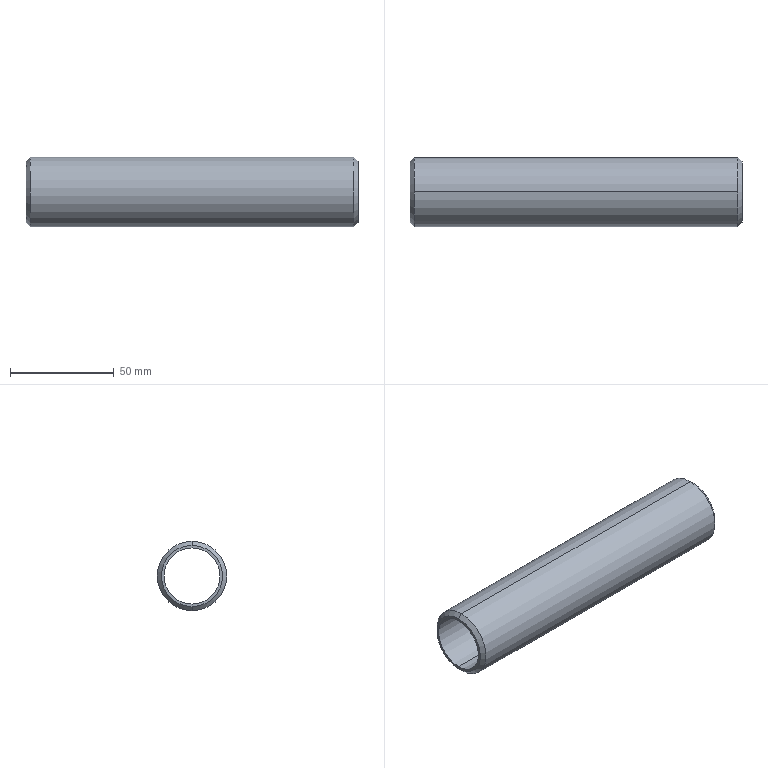Part | SolidWorks | features Chamfer 1, ExtruThin 1 | 1 solid | 10 faces | box 160 x 33.5 x 33.5 mm | volume 49013 mm3 | cone 4 | cylinder 4 | plane 2 | commonest cylinder face diameters 27 x2 33.5 x2
STEP:
#1=CARTESIAN_POINT('',(0.,0.,14.75));
#2=VERTEX_POINT('',#1);
#3=CARTESIAN_POINT('',(0.,0.,-14.75));
#4=VERTEX_POINT('',#3);
#5=CARTESIAN_POINT('',(0.,0.,0.));
#6=DIRECTION('',(-1.,0.,0.));
#7=DIRECTION('',(0.,0.,-1.));
#8=AXIS2_PLACEMENT_3D('',#5,#6,#7);
#9=CIRCLE('',#8,14.75);
#10=EDGE_CURVE('',#2,#4,#9,.T.);
#11=ORIENTED_EDGE('',*,*,#10,.F.);
#12=CARTESIAN_POINT('',(2.,0.,16.75));
#13=VERTEX_POINT('',#12);
#14=CARTESIAN_POINT('',(2.,0.,16.75));
#15=DIRECTION('',(0.7071,0.,0.7071));
#16=VECTOR('',#15,1000.);
#17=LINE('',#14,#16);
#18=EDGE_CURVE('',#2,#13,#17,.T.);
#19=ORIENTED_EDGE('',*,*,#18,.T.);
#20=CARTESIAN_POINT('',(2.,0.,-16.75));
#21=VERTEX_POINT('',#20);
#22=CARTESIAN_POINT('',(2.,0.,0.));
#23=DIRECTION('',(1.,0.,0.));
#24=DIRECTION('',(0.,0.,-1.));
#25=AXIS2_PLACEMENT_3D('',#22,#23,#24);
#26=CIRCLE('',#25,16.75);
#27=EDGE_CURVE('',#21,#13,#26,.T.);
#28=ORIENTED_EDGE('',*,*,#27,.F.);
#29=CARTESIAN_POINT('',(2.,0.,-16.75));
#30=DIRECTION('',(0.7071,0.,-0.7071));
#31=VECTOR('',#30,1000.);
#32=LINE('',#29,#31);
#33=EDGE_CURVE('',#4,#21,#32,.T.);
#34=ORIENTED_EDGE('',*,*,#33,.F.);
#35=EDGE_LOOP('',(#11,#19,#28,#34));
#36=FACE_OUTER_BOUND('',#35,.T.);
#37=CARTESIAN_POINT('',(2.,0.,0.));
#38=DIRECTION('',(1.,0.,0.));
#39=DIRECTION('',(0.,0.,-1.));
#40=AXIS2_PLACEMENT_3D('',#37,#38,#39);
#41=CONICAL_SURFACE('',#40,16.75,0.7854);
#42=ADVANCED_FACE('',(#36),#41,.T.);
#43=CARTESIAN_POINT('',(160.,0.,-14.75));
#44=VERTEX_POINT('',#43);
#45=CARTESIAN_POINT('',(160.,0.,14.75));
#46=VERTEX_POINT('',#45);
#47=CARTESIAN_POINT('',(160.,0.,0.));
#48=DIRECTION('',(1.,0.,0.));
#49=DIRECTION('',(0.,0.,-1.));
#50=AXIS2_PLACEMENT_3D('',#47,#48,#49);
#51=CIRCLE('',#50,14.75);
#52=EDGE_CURVE('',#44,#46,#51,.T.);
#53=ORIENTED_EDGE('',*,*,#52,.F.);
#54=CARTESIAN_POINT('',(158.,0.,-16.75));
#55=VERTEX_POINT('',#54);
#56=CARTESIAN_POINT('',(160.,0.,-14.75));
#57=DIRECTION('',(-0.7071,0.,-0.7071));
#58=VECTOR('',#57,1000.);
#59=LINE('',#56,#58);
#60=EDGE_CURVE('',#44,#55,#59,.T.);
#61=ORIENTED_EDGE('',*,*,#60,.T.);
#62=CARTESIAN_POINT('',(158.,0.,16.75));
#63=VERTEX_POINT('',#62);
#64=CARTESIAN_POINT('',(158.,0.,0.));
#65=DIRECTION('',(-1.,0.,0.));
#66=DIRECTION('',(0.,0.,-1.));
#67=AXIS2_PLACEMENT_3D('',#64,#65,#66);
#68=CIRCLE('',#67,16.75);
#69=EDGE_CURVE('',#63,#55,#68,.T.);
#70=ORIENTED_EDGE('',*,*,#69,.F.);
#71=CARTESIAN_POINT('',(160.,0.,14.75));
#72=DIRECTION('',(-0.7071,0.,0.7071));
#73=VECTOR('',#72,1000.);
#74=LINE('',#71,#73);
#75=EDGE_CURVE('',#46,#63,#74,.T.);
#76=ORIENTED_EDGE('',*,*,#75,.F.);
#77=EDGE_LOOP('',(#53,#61,#70,#76));
#78=FACE_OUTER_BOUND('',#77,.T.);
#79=CARTESIAN_POINT('',(160.,0.,0.));
#80=DIRECTION('',(-1.,0.,0.));
#81=DIRECTION('',(0.,0.,1.));
#82=AXIS2_PLACEMENT_3D('',#79,#80,#81);
#83=CONICAL_SURFACE('',#82,14.75,0.7854);
#84=ADVANCED_FACE('',(#78),#83,.T.);
#85=CARTESIAN_POINT('',(160.,0.,13.5));
#86=VERTEX_POINT('',#85);
#87=CARTESIAN_POINT('',(160.,0.,-13.5));
#88=VERTEX_POINT('',#87);
#89=CARTESIAN_POINT('',(160.,0.,0.));
#90=DIRECTION('',(1.,0.,0.));
#91=DIRECTION('',(0.,0.,-1.));
#92=AXIS2_PLACEMENT_3D('',#89,#90,#91);
#93=CIRCLE('',#92,13.5);
#94=EDGE_CURVE('',#86,#88,#93,.T.);
#95=ORIENTED_EDGE('',*,*,#94,.T.);
#96=CARTESIAN_POINT('',(0.,0.,-13.5));
#97=VERTEX_POINT('',#96);
#98=CARTESIAN_POINT('',(160.,0.,-13.5));
#99=DIRECTION('',(-1.,0.,0.));
#100=VECTOR('',#99,1000.);
#101=LINE('',#98,#100);
#102=EDGE_CURVE('',#88,#97,#101,.T.);
#103=ORIENTED_EDGE('',*,*,#102,.T.);
#104=CARTESIAN_POINT('',(0.,0.,13.5));
#105=VERTEX_POINT('',#104);
#106=CARTESIAN_POINT('',(0.,0.,0.));
#107=DIRECTION('',(1.,0.,0.));
#108=DIRECTION('',(0.,0.,-1.));
#109=AXIS2_PLACEMENT_3D('',#106,#107,#108);
#110=CIRCLE('',#109,13.5);
#111=EDGE_CURVE('',#105,#97,#110,.T.);
#112=ORIENTED_EDGE('',*,*,#111,.F.);
#113=CARTESIAN_POINT('',(160.,0.,13.5));
#114=DIRECTION('',(-1.,0.,0.));
#115=VECTOR('',#114,1000.);
#116=LINE('',#113,#115);
#117=EDGE_CURVE('',#86,#105,#116,.T.);
#118=ORIENTED_EDGE('',*,*,#117,.F.);
#119=EDGE_LOOP('',(#95,#103,#112,#118));
#120=FACE_OUTER_BOUND('',#119,.T.);
#121=CARTESIAN_POINT('',(160.,0.,0.));
#122=DIRECTION('',(-1.,0.,0.));
#123=DIRECTION('',(0.,0.,1.));
#124=AXIS2_PLACEMENT_3D('',#121,#122,#123);
#125=CYLINDRICAL_SURFACE('',#124,13.5);
#126=ADVANCED_FACE('',(#120),#125,.F.);
#127=ORIENTED_EDGE('',*,*,#69,.T.);
#128=CARTESIAN_POINT('',(160.,0.,-16.75));
#129=DIRECTION('',(-1.,0.,0.));
#130=VECTOR('',#129,1000.);
#131=LINE('',#128,#130);
#132=EDGE_CURVE('',#55,#21,#131,.T.);
#133=ORIENTED_EDGE('',*,*,#132,.T.);
#134=ORIENTED_EDGE('',*,*,#27,.T.);
#135=CARTESIAN_POINT('',(160.,0.,16.75));
#136=DIRECTION('',(-1.,0.,0.));
#137=VECTOR('',#136,1000.);
#138=LINE('',#135,#137);
#139=EDGE_CURVE('',#63,#13,#138,.T.);
#140=ORIENTED_EDGE('',*,*,#139,.F.);
#141=EDGE_LOOP('',(#127,#133,#134,#140));
#142=FACE_OUTER_BOUND('',#141,.T.);
#143=CARTESIAN_POINT('',(160.,0.,0.));
#144=DIRECTION('',(-1.,0.,0.));
#145=DIRECTION('',(0.,0.,1.));
#146=AXIS2_PLACEMENT_3D('',#143,#144,#145);
#147=CYLINDRICAL_SURFACE('',#146,16.75);
#148=ADVANCED_FACE('',(#142),#147,.T.);
#149=CARTESIAN_POINT('',(160.,0.,0.));
#150=DIRECTION('',(1.,0.,0.));
#151=DIRECTION('',(0.,0.,-1.));
#152=AXIS2_PLACEMENT_3D('',#149,#150,#151);
#153=CIRCLE('',#152,14.75);
#154=EDGE_CURVE('',#46,#44,#153,.T.);
#155=ORIENTED_EDGE('',*,*,#154,.T.);
#156=ORIENTED_EDGE('',*,*,#52,.T.);
#157=EDGE_LOOP('',(#155,#156));
#158=FACE_OUTER_BOUND('',#157,.T.);
#159=ORIENTED_EDGE('',*,*,#94,.F.);
#160=CARTESIAN_POINT('',(160.,0.,0.));
#161=DIRECTION('',(1.,0.,0.));
#162=DIRECTION('',(0.,0.,-1.));
#163=AXIS2_PLACEMENT_3D('',#160,#161,#162);
#164=CIRCLE('',#163,13.5);
#165=EDGE_CURVE('',#88,#86,#164,.T.);
#166=ORIENTED_EDGE('',*,*,#165,.F.);
#167=EDGE_LOOP('',(#159,#166));
#168=FACE_BOUND('',#167,.T.);
#169=CARTESIAN_POINT('',(160.,0.,0.));
#170=DIRECTION('',(1.,0.,0.));
#171=DIRECTION('',(0.,0.,-1.));
#172=AXIS2_PLACEMENT_3D('',#169,#170,#171);
#173=PLANE('',#172);
#174=ADVANCED_FACE('',(#158,#168),#173,.T.);
#175=CARTESIAN_POINT('',(0.,0.,0.));
#176=DIRECTION('',(-1.,0.,0.));
#177=DIRECTION('',(0.,0.,-1.));
#178=AXIS2_PLACEMENT_3D('',#175,#176,#177);
#179=CIRCLE('',#178,14.75);
#180=EDGE_CURVE('',#4,#2,#179,.T.);
#181=ORIENTED_EDGE('',*,*,#180,.T.);
#182=ORIENTED_EDGE('',*,*,#10,.T.);
#183=EDGE_LOOP('',(#181,#182));
#184=FACE_OUTER_BOUND('',#183,.T.);
#185=ORIENTED_EDGE('',*,*,#111,.T.);
#186=CARTESIAN_POINT('',(0.,0.,0.));
#187=DIRECTION('',(1.,0.,0.));
#188=DIRECTION('',(0.,0.,-1.));
#189=AXIS2_PLACEMENT_3D('',#186,#187,#188);
#190=CIRCLE('',#189,13.5);
#191=EDGE_CURVE('',#97,#105,#190,.T.);
#192=ORIENTED_EDGE('',*,*,#191,.T.);
#193=EDGE_LOOP('',(#185,#192));
#194=FACE_BOUND('',#193,.T.);
#195=CARTESIAN_POINT('',(0.,0.,0.));
#196=DIRECTION('',(1.,0.,0.));
#197=DIRECTION('',(0.,0.,-1.));
#198=AXIS2_PLACEMENT_3D('',#195,#196,#197);
#199=PLANE('',#198);
#200=ADVANCED_FACE('',(#184,#194),#199,.F.);
#201=ORIENTED_EDGE('',*,*,#132,.F.);
#202=CARTESIAN_POINT('',(158.,0.,0.));
#203=DIRECTION('',(-1.,0.,0.));
#204=DIRECTION('',(0.,0.,-1.));
#205=AXIS2_PLACEMENT_3D('',#202,#203,#204);
#206=CIRCLE('',#205,16.75);
#207=EDGE_CURVE('',#55,#63,#206,.T.);
#208=ORIENTED_EDGE('',*,*,#207,.T.);
#209=ORIENTED_EDGE('',*,*,#139,.T.);
#210=CARTESIAN_POINT('',(2.,0.,0.));
#211=DIRECTION('',(1.,0.,0.));
#212=DIRECTION('',(0.,0.,-1.));
#213=AXIS2_PLACEMENT_3D('',#210,#211,#212);
#214=CIRCLE('',#213,16.75);
#215=EDGE_CURVE('',#13,#21,#214,.T.);
#216=ORIENTED_EDGE('',*,*,#215,.T.);
#217=EDGE_LOOP('',(#201,#208,#209,#216));
#218=FACE_OUTER_BOUND('',#217,.T.);
#219=CARTESIAN_POINT('',(160.,0.,0.));
#220=DIRECTION('',(-1.,0.,0.));
#221=DIRECTION('',(0.,0.,1.));
#222=AXIS2_PLACEMENT_3D('',#219,#220,#221);
#223=CYLINDRICAL_SURFACE('',#222,16.75);
#224=ADVANCED_FACE('',(#218),#223,.T.);
#225=ORIENTED_EDGE('',*,*,#102,.F.);
#226=ORIENTED_EDGE('',*,*,#165,.T.);
#227=ORIENTED_EDGE('',*,*,#117,.T.);
#228=ORIENTED_EDGE('',*,*,#191,.F.);
#229=EDGE_LOOP('',(#225,#226,#227,#228));
#230=FACE_OUTER_BOUND('',#229,.T.);
#231=CARTESIAN_POINT('',(160.,0.,0.));
#232=DIRECTION('',(-1.,0.,0.));
#233=DIRECTION('',(0.,0.,1.));
#234=AXIS2_PLACEMENT_3D('',#231,#232,#233);
#235=CYLINDRICAL_SURFACE('',#234,13.5);
#236=ADVANCED_FACE('',(#230),#235,.F.);
#237=ORIENTED_EDGE('',*,*,#60,.F.);
#238=ORIENTED_EDGE('',*,*,#154,.F.);
#239=ORIENTED_EDGE('',*,*,#75,.T.);
#240=ORIENTED_EDGE('',*,*,#207,.F.);
#241=EDGE_LOOP('',(#237,#238,#239,#240));
#242=FACE_OUTER_BOUND('',#241,.T.);
#243=CARTESIAN_POINT('',(160.,0.,0.));
#244=DIRECTION('',(-1.,0.,0.));
#245=DIRECTION('',(0.,0.,1.));
#246=AXIS2_PLACEMENT_3D('',#243,#244,#245);
#247=CONICAL_SURFACE('',#246,14.75,0.7854);
#248=ADVANCED_FACE('',(#242),#247,.T.);
#249=ORIENTED_EDGE('',*,*,#18,.F.);
#250=ORIENTED_EDGE('',*,*,#180,.F.);
#251=ORIENTED_EDGE('',*,*,#33,.T.);
#252=ORIENTED_EDGE('',*,*,#215,.F.);
#253=EDGE_LOOP('',(#249,#250,#251,#252));
#254=FACE_OUTER_BOUND('',#253,.T.);
#255=CARTESIAN_POINT('',(2.,0.,0.));
#256=DIRECTION('',(1.,0.,0.));
#257=DIRECTION('',(0.,0.,-1.));
#258=AXIS2_PLACEMENT_3D('',#255,#256,#257);
#259=CONICAL_SURFACE('',#258,16.75,0.7854);
#260=ADVANCED_FACE('',(#254),#259,.T.);
#261=CLOSED_SHELL('',(#42,#84,#126,#148,#174,#200,#224,#236,#248,#260));
#262=MANIFOLD_SOLID_BREP('',#261);
#263=CARTESIAN_POINT('',(0.,0.,0.));
#264=DIRECTION('',(0.,0.,1.));
#265=DIRECTION('',(1.,0.,0.));
#266=AXIS2_PLACEMENT_3D('',#263,#264,#265);
#267=(LENGTH_UNIT()NAMED_UNIT(*)SI_UNIT(.MILLI.,.METRE.));
#268=UNCERTAINTY_MEASURE_WITH_UNIT(LENGTH_MEASURE(0.00001),#267,'','');
#269=(NAMED_UNIT(*)PLANE_ANGLE_UNIT()SI_UNIT($,.RADIAN.));
#270=(NAMED_UNIT(*)SI_UNIT($,.STERADIAN.)SOLID_ANGLE_UNIT());
#271=(GEOMETRIC_REPRESENTATION_CONTEXT(3)GLOBAL_UNCERTAINTY_ASSIGNED_CONTEXT((#268))GLOBAL_UNIT_ASSIGNED_CONTEXT((#267,#269,#270))REPRESENTATION_CONTEXT('',''));
#272=ADVANCED_BREP_SHAPE_REPRESENTATION('',(#262,#266),#271);